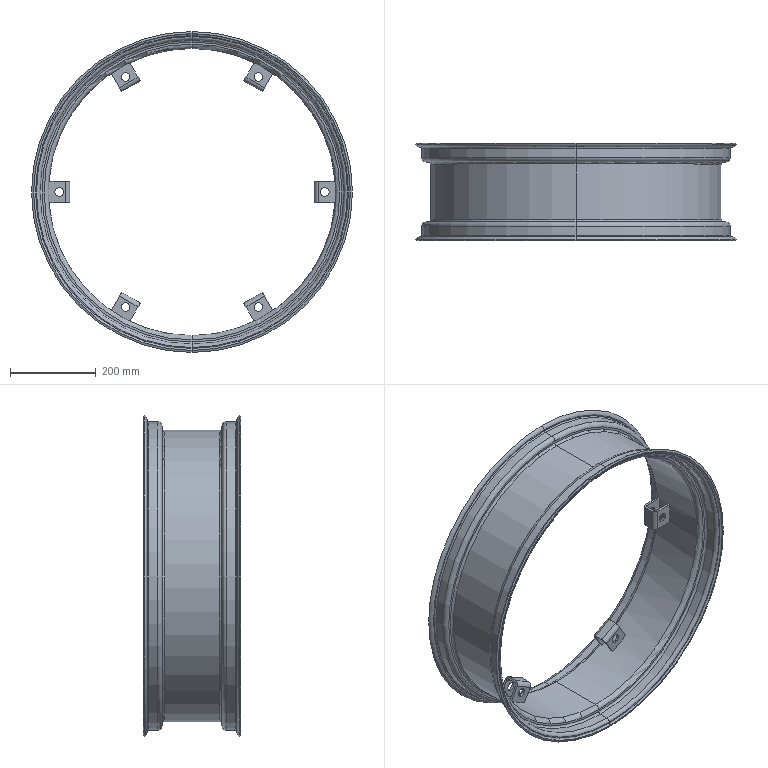Part | SolidWorks | 1 solid | 152 faces | box 748.86 x 226.672 x 748.86 mm | volume 3116761 mm3 | cylinder 60 | plane 56 | torus 32 | cone 4 | commonest cylinder face diameters 20 x36 10 x12 710 x4 720 x4 670 x2 680 x2